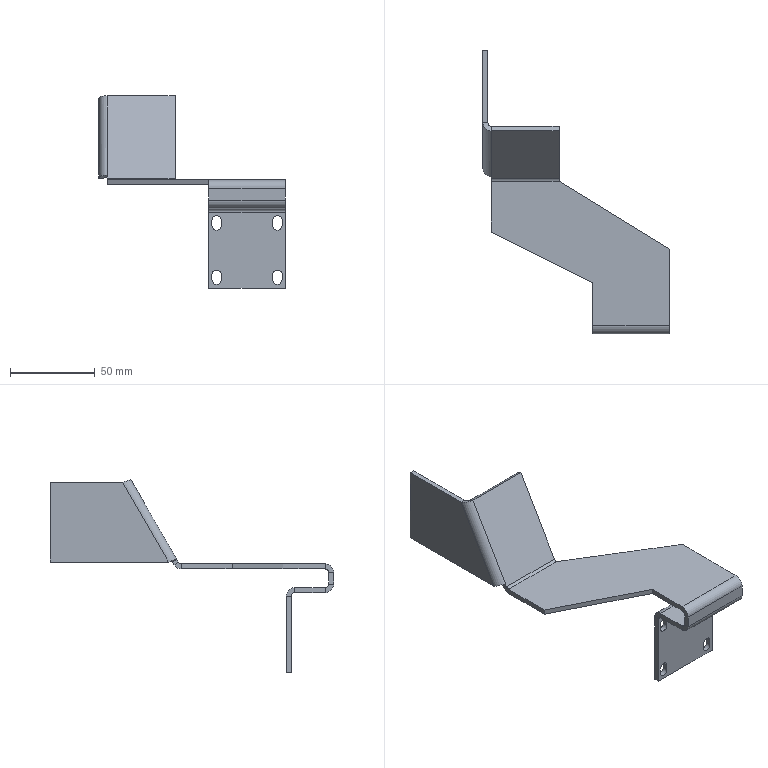Part | STEP file | Push-film plate SGN-3-09 | 1 solid | 70 faces | box 110 x 167.387 x 113.677 mm | volume 42869 mm3 | plane 46 | cylinder 22 | spline 2 | commonest cylinder face diameters 5.5 x12 4 x5 10 x5